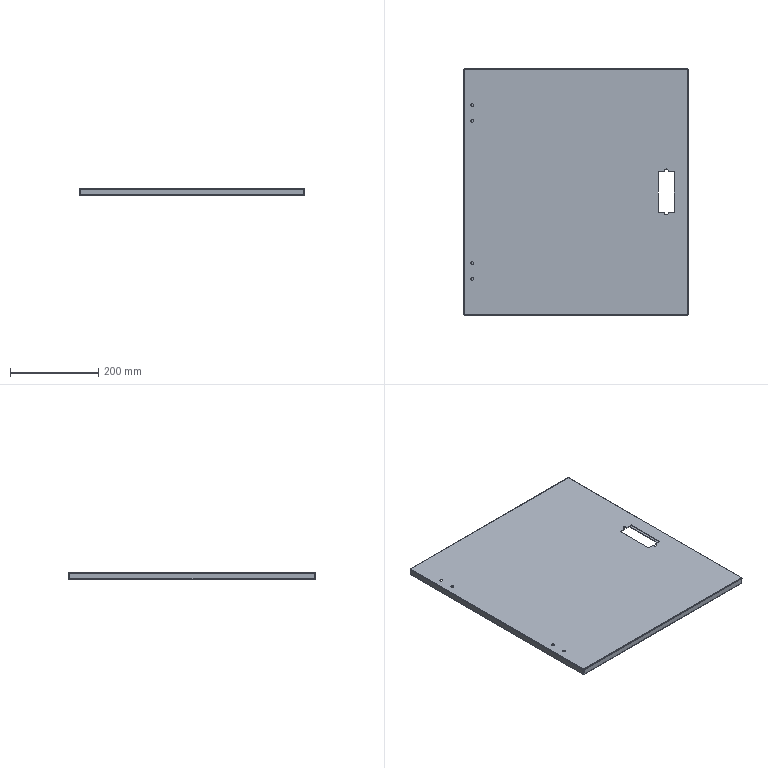Part | STEP file | Left door panel sheet metal_PN_0004 | 1 solid | 90 faces | box 508.5 x 557 x 15 mm | volume 531244 mm3 | plane 48 | cylinder 26 | spline 16 | commonest cylinder face diameters 0.2 x8 3.2 x8 6.5 x8 8 x2